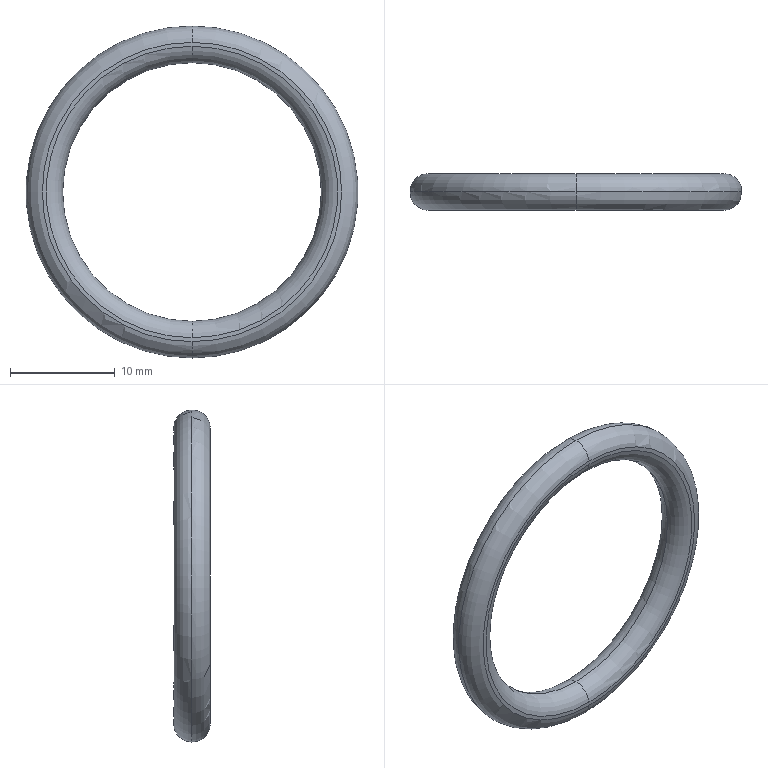Part | STEP file | PN_0002_default | 1 solid | 7 faces | box 31.7 x 3.49 x 31.7 mm | volume 852.143 mm3 | torus 6 | plane 1
STEP:
#1=CARTESIAN_POINT('',(0.,0.,0.));
#2=DIRECTION('',(0.,0.,1.));
#3=DIRECTION('',(1.,0.,0.));
#4=AXIS2_PLACEMENT_3D('',#1,#2,#3);
#5=CARTESIAN_POINT('',(0.,0.,-15.85));
#6=VERTEX_POINT('',#5);
#7=CARTESIAN_POINT('',(0.,0.,-12.35));
#8=VERTEX_POINT('',#7);
#9=CARTESIAN_POINT('',(0.,0.,-14.1));
#10=DIRECTION('',(1.,0.,0.));
#11=DIRECTION('',(0.,0.,-1.));
#12=AXIS2_PLACEMENT_3D('',#9,#10,#11);
#13=CIRCLE('',#12,1.75);
#14=CARTESIAN_POINT('',(0.,0.,0.));
#15=DIRECTION('',(0.,1.,0.));
#16=DIRECTION('',(0.,0.,1.));
#17=AXIS2_PLACEMENT_3D('',#14,#15,#16);
#18=TOROIDAL_SURFACE('',#17,14.1,1.75);
#19=CARTESIAN_POINT('',(3.142,0.));
#20=DIRECTION('',(0.,1.));
#21=VECTOR('',#20,1.);
#22=LINE('',#19,#21);
#23=(GEOMETRIC_REPRESENTATION_CONTEXT(2)PARAMETRIC_REPRESENTATION_CONTEXT()REPRESENTATION_CONTEXT('',''));
#24=DEFINITIONAL_REPRESENTATION('',(#22),#23);
#25=PCURVE('',#18,#24);
#26=CARTESIAN_POINT('',(0.,0.,0.));
#27=DIRECTION('',(0.,1.,0.));
#28=DIRECTION('',(0.,0.,1.));
#29=AXIS2_PLACEMENT_3D('',#26,#27,#28);
#30=TOROIDAL_SURFACE('',#29,14.1,1.75);
#31=CARTESIAN_POINT('',(3.142,0.));
#32=DIRECTION('',(0.,1.));
#33=VECTOR('',#32,1.);
#34=LINE('',#31,#33);
#35=(GEOMETRIC_REPRESENTATION_CONTEXT(2)PARAMETRIC_REPRESENTATION_CONTEXT()REPRESENTATION_CONTEXT('',''));
#36=DEFINITIONAL_REPRESENTATION('',(#34),#35);
#37=PCURVE('',#30,#36);
#38=SURFACE_CURVE('',#13,(#25,#37),.PCURVE_S1.);
#39=EDGE_CURVE('',#6,#8,#38,.T.);
#40=ORIENTED_EDGE('',*,*,#39,.F.);
#41=CARTESIAN_POINT('',(0.,0.,15.85));
#42=VERTEX_POINT('',#41);
#43=CARTESIAN_POINT('',(0.,0.,0.));
#44=DIRECTION('',(0.,1.,0.));
#45=DIRECTION('',(0.,0.,1.));
#46=AXIS2_PLACEMENT_3D('',#43,#44,#45);
#47=CIRCLE('',#46,15.85);
#48=CARTESIAN_POINT('',(0.,0.));
#49=DIRECTION('',(1.,0.));
#50=VECTOR('',#49,1.);
#51=LINE('',#48,#50);
#52=(GEOMETRIC_REPRESENTATION_CONTEXT(2)PARAMETRIC_REPRESENTATION_CONTEXT()REPRESENTATION_CONTEXT('',''));
#53=DEFINITIONAL_REPRESENTATION('',(#51),#52);
#54=PCURVE('',#18,#53);
#55=CARTESIAN_POINT('',(0.,0.,0.));
#56=DIRECTION('',(0.,1.,0.));
#57=DIRECTION('',(0.,0.,1.));
#58=AXIS2_PLACEMENT_3D('',#55,#56,#57);
#59=TOROIDAL_SURFACE('',#58,14.1,1.75);
#60=CARTESIAN_POINT('',(0.,6.283));
#61=DIRECTION('',(1.,0.));
#62=VECTOR('',#61,1.);
#63=LINE('',#60,#62);
#64=(GEOMETRIC_REPRESENTATION_CONTEXT(2)PARAMETRIC_REPRESENTATION_CONTEXT()REPRESENTATION_CONTEXT('',''));
#65=DEFINITIONAL_REPRESENTATION('',(#63),#64);
#66=PCURVE('',#59,#65);
#67=SURFACE_CURVE('',#47,(#54,#66),.PCURVE_S1.);
#68=EDGE_CURVE('',#6,#42,#67,.T.);
#69=ORIENTED_EDGE('',*,*,#68,.T.);
#70=CARTESIAN_POINT('',(0.,0.,12.35));
#71=VERTEX_POINT('',#70);
#72=CARTESIAN_POINT('',(0.,0.,14.1));
#73=DIRECTION('',(-1.,0.,0.));
#74=DIRECTION('',(0.,0.,1.));
#75=AXIS2_PLACEMENT_3D('',#72,#73,#74);
#76=CIRCLE('',#75,1.75);
#77=CARTESIAN_POINT('',(6.283,0.));
#78=DIRECTION('',(0.,1.));
#79=VECTOR('',#78,1.);
#80=LINE('',#77,#79);
#81=(GEOMETRIC_REPRESENTATION_CONTEXT(2)PARAMETRIC_REPRESENTATION_CONTEXT()REPRESENTATION_CONTEXT('',''));
#82=DEFINITIONAL_REPRESENTATION('',(#80),#81);
#83=PCURVE('',#18,#82);
#84=CARTESIAN_POINT('',(0.,0.));
#85=DIRECTION('',(0.,1.));
#86=VECTOR('',#85,1.);
#87=LINE('',#84,#86);
#88=(GEOMETRIC_REPRESENTATION_CONTEXT(2)PARAMETRIC_REPRESENTATION_CONTEXT()REPRESENTATION_CONTEXT('',''));
#89=DEFINITIONAL_REPRESENTATION('',(#87),#88);
#90=PCURVE('',#30,#89);
#91=SURFACE_CURVE('',#76,(#83,#90),.PCURVE_S1.);
#92=EDGE_CURVE('',#42,#71,#91,.T.);
#93=ORIENTED_EDGE('',*,*,#92,.T.);
#94=CARTESIAN_POINT('',(0.,0.,0.));
#95=DIRECTION('',(0.,1.,0.));
#96=DIRECTION('',(0.,0.,1.));
#97=AXIS2_PLACEMENT_3D('',#94,#95,#96);
#98=CIRCLE('',#97,12.35);
#99=CARTESIAN_POINT('',(0.,3.142));
#100=DIRECTION('',(1.,0.));
#101=VECTOR('',#100,1.);
#102=LINE('',#99,#101);
#103=(GEOMETRIC_REPRESENTATION_CONTEXT(2)PARAMETRIC_REPRESENTATION_CONTEXT()REPRESENTATION_CONTEXT('',''));
#104=DEFINITIONAL_REPRESENTATION('',(#102),#103);
#105=PCURVE('',#18,#104);
#106=CARTESIAN_POINT('',(0.,0.,0.));
#107=DIRECTION('',(0.,1.,0.));
#108=DIRECTION('',(0.,0.,1.));
#109=AXIS2_PLACEMENT_3D('',#106,#107,#108);
#110=TOROIDAL_SURFACE('',#109,14.1,1.75);
#111=CARTESIAN_POINT('',(0.,3.142));
#112=DIRECTION('',(1.,0.));
#113=VECTOR('',#112,1.);
#114=LINE('',#111,#113);
#115=(GEOMETRIC_REPRESENTATION_CONTEXT(2)PARAMETRIC_REPRESENTATION_CONTEXT()REPRESENTATION_CONTEXT('',''));
#116=DEFINITIONAL_REPRESENTATION('',(#114),#115);
#117=PCURVE('',#110,#116);
#118=SURFACE_CURVE('',#98,(#105,#117),.PCURVE_S1.);
#119=EDGE_CURVE('',#8,#71,#118,.T.);
#120=ORIENTED_EDGE('',*,*,#119,.F.);
#121=EDGE_LOOP('',(#40,#69,#93,#120));
#122=FACE_BOUND('',#121,.T.);
#123=ADVANCED_FACE('',(#122),#18,.T.);
#124=CARTESIAN_POINT('',(0.,-1.74,-13.913));
#125=VERTEX_POINT('',#124);
#126=CARTESIAN_POINT('',(0.,0.,-14.1));
#127=DIRECTION('',(1.,0.,0.));
#128=DIRECTION('',(0.,0.,-1.));
#129=AXIS2_PLACEMENT_3D('',#126,#127,#128);
#130=CIRCLE('',#129,1.75);
#131=CARTESIAN_POINT('',(3.142,0.));
#132=DIRECTION('',(0.,1.));
#133=VECTOR('',#132,1.);
#134=LINE('',#131,#133);
#135=(GEOMETRIC_REPRESENTATION_CONTEXT(2)PARAMETRIC_REPRESENTATION_CONTEXT()REPRESENTATION_CONTEXT('',''));
#136=DEFINITIONAL_REPRESENTATION('',(#134),#135);
#137=PCURVE('',#110,#136);
#138=CARTESIAN_POINT('',(0.,0.,0.));
#139=DIRECTION('',(0.,1.,0.));
#140=DIRECTION('',(0.,0.,1.));
#141=AXIS2_PLACEMENT_3D('',#138,#139,#140);
#142=TOROIDAL_SURFACE('',#141,14.1,1.75);
#143=CARTESIAN_POINT('',(3.142,0.));
#144=DIRECTION('',(0.,1.));
#145=VECTOR('',#144,1.);
#146=LINE('',#143,#145);
#147=(GEOMETRIC_REPRESENTATION_CONTEXT(2)PARAMETRIC_REPRESENTATION_CONTEXT()REPRESENTATION_CONTEXT('',''));
#148=DEFINITIONAL_REPRESENTATION('',(#146),#147);
#149=PCURVE('',#142,#148);
#150=SURFACE_CURVE('',#130,(#137,#149),.PCURVE_S1.);
#151=EDGE_CURVE('',#8,#125,#150,.T.);
#152=ORIENTED_EDGE('',*,*,#151,.F.);
#153=ORIENTED_EDGE('',*,*,#119,.T.);
#154=CARTESIAN_POINT('',(0.,-1.74,13.913));
#155=VERTEX_POINT('',#154);
#156=CARTESIAN_POINT('',(0.,0.,14.1));
#157=DIRECTION('',(-1.,0.,0.));
#158=DIRECTION('',(0.,0.,1.));
#159=AXIS2_PLACEMENT_3D('',#156,#157,#158);
#160=CIRCLE('',#159,1.75);
#161=CARTESIAN_POINT('',(6.283,0.));
#162=DIRECTION('',(0.,1.));
#163=VECTOR('',#162,1.);
#164=LINE('',#161,#163);
#165=(GEOMETRIC_REPRESENTATION_CONTEXT(2)PARAMETRIC_REPRESENTATION_CONTEXT()REPRESENTATION_CONTEXT('',''));
#166=DEFINITIONAL_REPRESENTATION('',(#164),#165);
#167=PCURVE('',#110,#166);
#168=CARTESIAN_POINT('',(0.,0.));
#169=DIRECTION('',(0.,1.));
#170=VECTOR('',#169,1.);
#171=LINE('',#168,#170);
#172=(GEOMETRIC_REPRESENTATION_CONTEXT(2)PARAMETRIC_REPRESENTATION_CONTEXT()REPRESENTATION_CONTEXT('',''));
#173=DEFINITIONAL_REPRESENTATION('',(#171),#172);
#174=PCURVE('',#142,#173);
#175=SURFACE_CURVE('',#160,(#167,#174),.PCURVE_S1.);
#176=EDGE_CURVE('',#71,#155,#175,.T.);
#177=ORIENTED_EDGE('',*,*,#176,.T.);
#178=CARTESIAN_POINT('',(0.,-1.74,0.));
#179=DIRECTION('',(0.,1.,0.));
#180=DIRECTION('',(0.,0.,1.));
#181=AXIS2_PLACEMENT_3D('',#178,#179,#180);
#182=CIRCLE('',#181,13.913);
#183=CARTESIAN_POINT('',(0.,4.605));
#184=DIRECTION('',(1.,0.));
#185=VECTOR('',#184,1.);
#186=LINE('',#183,#185);
#187=(GEOMETRIC_REPRESENTATION_CONTEXT(2)PARAMETRIC_REPRESENTATION_CONTEXT()REPRESENTATION_CONTEXT('',''));
#188=DEFINITIONAL_REPRESENTATION('',(#186),#187);
#189=PCURVE('',#110,#188);
#190=CARTESIAN_POINT('',(13.913,-1.74,0.));
#191=DIRECTION('',(0.,1.,0.));
#192=DIRECTION('',(0.,0.,1.));
#193=AXIS2_PLACEMENT_3D('',#190,#191,#192);
#194=PLANE('',#193);
#195=CARTESIAN_POINT('',(0.,-13.913));
#196=DIRECTION('',(1.,0.));
#197=AXIS2_PLACEMENT_2D('',#195,#196);
#198=CIRCLE('',#197,13.913);
#199=(GEOMETRIC_REPRESENTATION_CONTEXT(2)PARAMETRIC_REPRESENTATION_CONTEXT()REPRESENTATION_CONTEXT('',''));
#200=DEFINITIONAL_REPRESENTATION('',(#198),#199);
#201=PCURVE('',#194,#200);
#202=SURFACE_CURVE('',#182,(#189,#201),.PCURVE_S1.);
#203=EDGE_CURVE('',#125,#155,#202,.T.);
#204=ORIENTED_EDGE('',*,*,#203,.F.);
#205=EDGE_LOOP('',(#152,#153,#177,#204));
#206=FACE_BOUND('',#205,.T.);
#207=ADVANCED_FACE('',(#206),#110,.T.);
#208=ORIENTED_EDGE('',*,*,#92,.F.);
#209=CARTESIAN_POINT('',(0.,0.,0.));
#210=DIRECTION('',(0.,1.,0.));
#211=DIRECTION('',(0.,0.,1.));
#212=AXIS2_PLACEMENT_3D('',#209,#210,#211);
#213=CIRCLE('',#212,15.85);
#214=CARTESIAN_POINT('',(0.,0.));
#215=DIRECTION('',(1.,0.));
#216=VECTOR('',#215,1.);
#217=LINE('',#214,#216);
#218=(GEOMETRIC_REPRESENTATION_CONTEXT(2)PARAMETRIC_REPRESENTATION_CONTEXT()REPRESENTATION_CONTEXT('',''));
#219=DEFINITIONAL_REPRESENTATION('',(#217),#218);
#220=PCURVE('',#30,#219);
#221=CARTESIAN_POINT('',(0.,0.,0.));
#222=DIRECTION('',(0.,1.,0.));
#223=DIRECTION('',(0.,0.,1.));
#224=AXIS2_PLACEMENT_3D('',#221,#222,#223);
#225=TOROIDAL_SURFACE('',#224,14.1,1.75);
#226=CARTESIAN_POINT('',(0.,6.283));
#227=DIRECTION('',(1.,0.));
#228=VECTOR('',#227,1.);
#229=LINE('',#226,#228);
#230=(GEOMETRIC_REPRESENTATION_CONTEXT(2)PARAMETRIC_REPRESENTATION_CONTEXT()REPRESENTATION_CONTEXT('',''));
#231=DEFINITIONAL_REPRESENTATION('',(#229),#230);
#232=PCURVE('',#225,#231);
#233=SURFACE_CURVE('',#213,(#220,#232),.PCURVE_S1.);
#234=EDGE_CURVE('',#42,#6,#233,.T.);
#235=ORIENTED_EDGE('',*,*,#234,.T.);
#236=ORIENTED_EDGE('',*,*,#39,.T.);
#237=CARTESIAN_POINT('',(0.,0.,0.));
#238=DIRECTION('',(0.,1.,0.));
#239=DIRECTION('',(0.,0.,1.));
#240=AXIS2_PLACEMENT_3D('',#237,#238,#239);
#241=CIRCLE('',#240,12.35);
#242=CARTESIAN_POINT('',(0.,3.142));
#243=DIRECTION('',(1.,0.));
#244=VECTOR('',#243,1.);
#245=LINE('',#242,#244);
#246=(GEOMETRIC_REPRESENTATION_CONTEXT(2)PARAMETRIC_REPRESENTATION_CONTEXT()REPRESENTATION_CONTEXT('',''));
#247=DEFINITIONAL_REPRESENTATION('',(#245),#246);
#248=PCURVE('',#30,#247);
#249=CARTESIAN_POINT('',(0.,3.142));
#250=DIRECTION('',(1.,0.));
#251=VECTOR('',#250,1.);
#252=LINE('',#249,#251);
#253=(GEOMETRIC_REPRESENTATION_CONTEXT(2)PARAMETRIC_REPRESENTATION_CONTEXT()REPRESENTATION_CONTEXT('',''));
#254=DEFINITIONAL_REPRESENTATION('',(#252),#253);
#255=PCURVE('',#142,#254);
#256=SURFACE_CURVE('',#241,(#248,#255),.PCURVE_S1.);
#257=EDGE_CURVE('',#71,#8,#256,.T.);
#258=ORIENTED_EDGE('',*,*,#257,.F.);
#259=EDGE_LOOP('',(#208,#235,#236,#258));
#260=FACE_BOUND('',#259,.T.);
#261=ADVANCED_FACE('',(#260),#30,.T.);
#262=ORIENTED_EDGE('',*,*,#176,.F.);
#263=ORIENTED_EDGE('',*,*,#257,.T.);
#264=ORIENTED_EDGE('',*,*,#151,.T.);
#265=CARTESIAN_POINT('',(0.,-1.74,0.));
#266=DIRECTION('',(0.,1.,0.));
#267=DIRECTION('',(0.,0.,1.));
#268=AXIS2_PLACEMENT_3D('',#265,#266,#267);
#269=CIRCLE('',#268,13.913);
#270=CARTESIAN_POINT('',(0.,4.605));
#271=DIRECTION('',(1.,0.));
#272=VECTOR('',#271,1.);
#273=LINE('',#270,#272);
#274=(GEOMETRIC_REPRESENTATION_CONTEXT(2)PARAMETRIC_REPRESENTATION_CONTEXT()REPRESENTATION_CONTEXT('',''));
#275=DEFINITIONAL_REPRESENTATION('',(#273),#274);
#276=PCURVE('',#142,#275);
#277=CARTESIAN_POINT('',(0.,-13.913));
#278=DIRECTION('',(1.,0.));
#279=AXIS2_PLACEMENT_2D('',#277,#278);
#280=CIRCLE('',#279,13.913);
#281=(GEOMETRIC_REPRESENTATION_CONTEXT(2)PARAMETRIC_REPRESENTATION_CONTEXT()REPRESENTATION_CONTEXT('',''));
#282=DEFINITIONAL_REPRESENTATION('',(#280),#281);
#283=PCURVE('',#194,#282);
#284=SURFACE_CURVE('',#269,(#276,#283),.PCURVE_S1.);
#285=EDGE_CURVE('',#155,#125,#284,.T.);
#286=ORIENTED_EDGE('',*,*,#285,.F.);
#287=EDGE_LOOP('',(#262,#263,#264,#286));
#288=FACE_BOUND('',#287,.T.);
#289=ADVANCED_FACE('',(#288),#142,.T.);
#290=ORIENTED_EDGE('',*,*,#234,.F.);
#291=CARTESIAN_POINT('',(0.,-1.74,14.287));
#292=VERTEX_POINT('',#291);
#293=CARTESIAN_POINT('',(0.,0.,14.1));
#294=DIRECTION('',(-1.,0.,0.));
#295=DIRECTION('',(0.,0.,1.));
#296=AXIS2_PLACEMENT_3D('',#293,#294,#295);
#297=CIRCLE('',#296,1.75);
#298=CARTESIAN_POINT('',(0.,0.));
#299=DIRECTION('',(0.,1.));
#300=VECTOR('',#299,1.);
#301=LINE('',#298,#300);
#302=(GEOMETRIC_REPRESENTATION_CONTEXT(2)PARAMETRIC_REPRESENTATION_CONTEXT()REPRESENTATION_CONTEXT('',''));
#303=DEFINITIONAL_REPRESENTATION('',(#301),#302);
#304=PCURVE('',#225,#303);
#305=CARTESIAN_POINT('',(6.283,0.));
#306=DIRECTION('',(0.,1.));
#307=VECTOR('',#306,1.);
#308=LINE('',#305,#307);
#309=(GEOMETRIC_REPRESENTATION_CONTEXT(2)PARAMETRIC_REPRESENTATION_CONTEXT()REPRESENTATION_CONTEXT('',''));
#310=DEFINITIONAL_REPRESENTATION('',(#308),#309);
#311=PCURVE('',#59,#310);
#312=SURFACE_CURVE('',#297,(#304,#311),.PCURVE_S1.);
#313=EDGE_CURVE('',#292,#42,#312,.T.);
#314=ORIENTED_EDGE('',*,*,#313,.F.);
#315=CARTESIAN_POINT('',(0.,-1.74,-14.287));
#316=VERTEX_POINT('',#315);
#317=CARTESIAN_POINT('',(0.,-1.74,0.));
#318=DIRECTION('',(0.,1.,0.));
#319=DIRECTION('',(0.,0.,1.));
#320=AXIS2_PLACEMENT_3D('',#317,#318,#319);
#321=CIRCLE('',#320,14.287);
#322=CARTESIAN_POINT('',(0.,4.819));
#323=DIRECTION('',(1.,0.));
#324=VECTOR('',#323,1.);
#325=LINE('',#322,#324);
#326=(GEOMETRIC_REPRESENTATION_CONTEXT(2)PARAMETRIC_REPRESENTATION_CONTEXT()REPRESENTATION_CONTEXT('',''));
#327=DEFINITIONAL_REPRESENTATION('',(#325),#326);
#328=PCURVE('',#225,#327);
#329=CARTESIAN_POINT('',(0.,-13.913));
#330=DIRECTION('',(1.,0.));
#331=AXIS2_PLACEMENT_2D('',#329,#330);
#332=CIRCLE('',#331,14.287);
#333=(GEOMETRIC_REPRESENTATION_CONTEXT(2)PARAMETRIC_REPRESENTATION_CONTEXT()REPRESENTATION_CONTEXT('',''));
#334=DEFINITIONAL_REPRESENTATION('',(#332),#333);
#335=PCURVE('',#194,#334);
#336=SURFACE_CURVE('',#321,(#328,#335),.PCURVE_S1.);
#337=EDGE_CURVE('',#292,#316,#336,.T.);
#338=ORIENTED_EDGE('',*,*,#337,.T.);
#339=CARTESIAN_POINT('',(0.,0.,-14.1));
#340=DIRECTION('',(1.,0.,0.));
#341=DIRECTION('',(0.,0.,-1.));
#342=AXIS2_PLACEMENT_3D('',#339,#340,#341);
#343=CIRCLE('',#342,1.75);
#344=CARTESIAN_POINT('',(3.142,0.));
#345=DIRECTION('',(0.,1.));
#346=VECTOR('',#345,1.);
#347=LINE('',#344,#346);
#348=(GEOMETRIC_REPRESENTATION_CONTEXT(2)PARAMETRIC_REPRESENTATION_CONTEXT()REPRESENTATION_CONTEXT('',''));
#349=DEFINITIONAL_REPRESENTATION('',(#347),#348);
#350=PCURVE('',#225,#349);
#351=CARTESIAN_POINT('',(3.142,0.));
#352=DIRECTION('',(0.,1.));
#353=VECTOR('',#352,1.);
#354=LINE('',#351,#353);
#355=(GEOMETRIC_REPRESENTATION_CONTEXT(2)PARAMETRIC_REPRESENTATION_CONTEXT()REPRESENTATION_CONTEXT('',''));
#356=DEFINITIONAL_REPRESENTATION('',(#354),#355);
#357=PCURVE('',#59,#356);
#358=SURFACE_CURVE('',#343,(#350,#357),.PCURVE_S1.);
#359=EDGE_CURVE('',#316,#6,#358,.T.);
#360=ORIENTED_EDGE('',*,*,#359,.T.);
#361=EDGE_LOOP('',(#290,#314,#338,#360));
#362=FACE_BOUND('',#361,.T.);
#363=ADVANCED_FACE('',(#362),#225,.T.);
#364=ORIENTED_EDGE('',*,*,#68,.F.);
#365=ORIENTED_EDGE('',*,*,#359,.F.);
#366=CARTESIAN_POINT('',(0.,-1.74,0.));
#367=DIRECTION('',(0.,1.,0.));
#368=DIRECTION('',(0.,0.,1.));
#369=AXIS2_PLACEMENT_3D('',#366,#367,#368);
#370=CIRCLE('',#369,14.287);
#371=CARTESIAN_POINT('',(0.,4.819));
#372=DIRECTION('',(1.,0.));
#373=VECTOR('',#372,1.);
#374=LINE('',#371,#373);
#375=(GEOMETRIC_REPRESENTATION_CONTEXT(2)PARAMETRIC_REPRESENTATION_CONTEXT()REPRESENTATION_CONTEXT('',''));
#376=DEFINITIONAL_REPRESENTATION('',(#374),#375);
#377=PCURVE('',#59,#376);
#378=CARTESIAN_POINT('',(0.,-13.913));
#379=DIRECTION('',(1.,0.));
#380=AXIS2_PLACEMENT_2D('',#378,#379);
#381=CIRCLE('',#380,14.287);
#382=(GEOMETRIC_REPRESENTATION_CONTEXT(2)PARAMETRIC_REPRESENTATION_CONTEXT()REPRESENTATION_CONTEXT('',''));
#383=DEFINITIONAL_REPRESENTATION('',(#381),#382);
#384=PCURVE('',#194,#383);
#385=SURFACE_CURVE('',#370,(#377,#384),.PCURVE_S1.);
#386=EDGE_CURVE('',#316,#292,#385,.T.);
#387=ORIENTED_EDGE('',*,*,#386,.T.);
#388=ORIENTED_EDGE('',*,*,#313,.T.);
#389=EDGE_LOOP('',(#364,#365,#387,#388));
#390=FACE_BOUND('',#389,.T.);
#391=ADVANCED_FACE('',(#390),#59,.T.);
#392=ORIENTED_EDGE('',*,*,#337,.F.);
#393=ORIENTED_EDGE('',*,*,#386,.F.);
#394=EDGE_LOOP('',(#392,#393));
#395=FACE_BOUND('',#394,.T.);
#396=ORIENTED_EDGE('',*,*,#285,.T.);
#397=ORIENTED_EDGE('',*,*,#203,.T.);
#398=EDGE_LOOP('',(#396,#397));
#399=FACE_BOUND('',#398,.T.);
#400=ADVANCED_FACE('',(#395,#399),#194,.F.);
#401=CLOSED_SHELL('',(#123,#207,#261,#289,#363,#391,#400));
#402=MANIFOLD_SOLID_BREP('',#401);
#403=(LENGTH_UNIT()NAMED_UNIT(*)SI_UNIT(.MILLI.,.METRE.));
#404=UNCERTAINTY_MEASURE_WITH_UNIT(LENGTH_MEASURE(0.0000001),#403,'','');
#405=(NAMED_UNIT(*)PLANE_ANGLE_UNIT()SI_UNIT($,.RADIAN.));
#406=(NAMED_UNIT(*)SI_UNIT($,.STERADIAN.)SOLID_ANGLE_UNIT());
#407=(GEOMETRIC_REPRESENTATION_CONTEXT(3)GLOBAL_UNCERTAINTY_ASSIGNED_CONTEXT((#404))GLOBAL_UNIT_ASSIGNED_CONTEXT((#403,#405,#406))REPRESENTATION_CONTEXT('',''));
#408=ADVANCED_BREP_SHAPE_REPRESENTATION('',(#4,#402),#407);